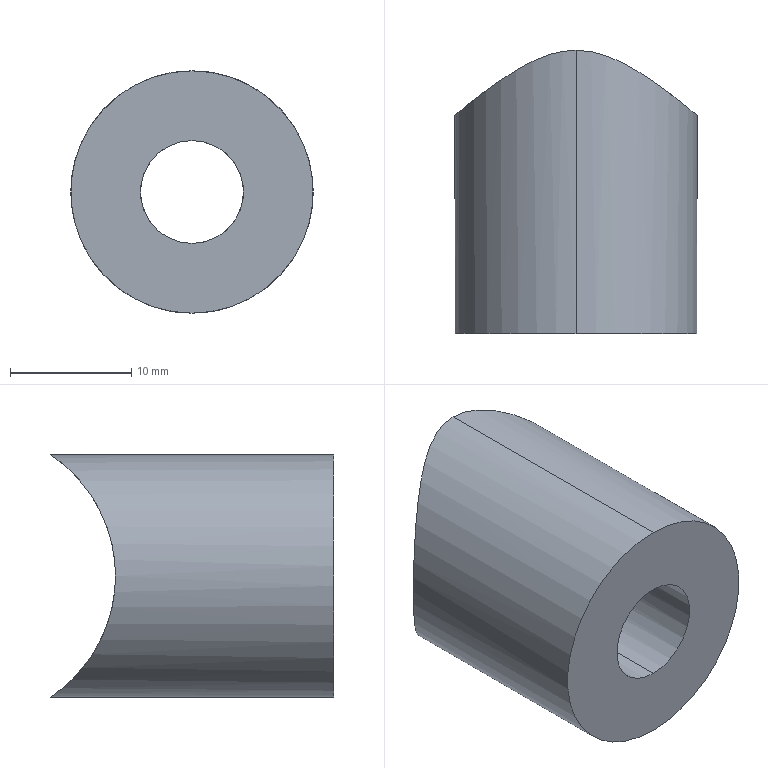Part | SolidWorks | features 3DProfileFeature 1, Extrusion 1, HoleWzd 1 | 1 solid | 7 faces | box 20 x 23.367 x 20 mm | volume 4988 mm3 | cylinder 6 | plane 1 | commonest cylinder face diameters 8.5 x2 20 x2 24 x2
STEP:
#1=CARTESIAN_POINT('',(-608.25,85.2,0.));
#2=VERTEX_POINT('',#1);
#3=CARTESIAN_POINT('',(-604.,85.978,4.25));
#4=VERTEX_POINT('',#3);
#5=CARTESIAN_POINT('',(-608.25,85.2,0.));
#6=CARTESIAN_POINT('',(-608.25,85.2,0.2798));
#7=CARTESIAN_POINT('',(-608.222,85.21,0.5639));
#8=CARTESIAN_POINT('',(-608.112,85.248,1.111));
#9=CARTESIAN_POINT('',(-608.031,85.276,1.377));
#10=CARTESIAN_POINT('',(-607.815,85.348,1.895));
#11=CARTESIAN_POINT('',(-607.683,85.39,2.139));
#12=CARTESIAN_POINT('',(-607.376,85.482,2.597));
#13=CARTESIAN_POINT('',(-607.198,85.533,2.813));
#14=CARTESIAN_POINT('',(-606.807,85.634,3.203));
#15=CARTESIAN_POINT('',(-606.595,85.684,3.377));
#16=CARTESIAN_POINT('',(-606.136,85.779,3.685));
#17=CARTESIAN_POINT('',(-605.887,85.823,3.818));
#18=CARTESIAN_POINT('',(-605.376,85.897,4.03));
#19=CARTESIAN_POINT('',(-605.111,85.926,4.112));
#20=CARTESIAN_POINT('',(-604.56,85.967,4.222));
#21=CARTESIAN_POINT('',(-604.279,85.978,4.25));
#22=CARTESIAN_POINT('',(-604.,85.978,4.25));
#23=B_SPLINE_CURVE_WITH_KNOTS('',3,(#5,#6,#7,#8,#9,#10,#11,#12,#13,#14,#15,#16,#17,#18,#19,#20,#21,#22),.UNSPECIFIED.,.F.,.F.,(4,2,2,2,2,2,2,2,4),(0.0067,0.007537,0.008374,0.009211,0.01005,0.01089,0.01172,0.01256,0.0134),.UNSPECIFIED.);
#24=EDGE_CURVE('',#2,#4,#23,.T.);
#25=ORIENTED_EDGE('',*,*,#24,.T.);
#26=CARTESIAN_POINT('',(-604.,67.2,4.25));
#27=VERTEX_POINT('',#26);
#28=CARTESIAN_POINT('',(-604.,67.2,4.25));
#29=DIRECTION('',(0.,-1.,0.));
#30=VECTOR('',#29,1000.);
#31=LINE('',#28,#30);
#32=EDGE_CURVE('',#4,#27,#31,.T.);
#33=ORIENTED_EDGE('',*,*,#32,.T.);
#34=CARTESIAN_POINT('',(-604.,67.2,-4.25));
#35=VERTEX_POINT('',#34);
#36=CARTESIAN_POINT('',(-604.,67.2,0.));
#37=DIRECTION('',(0.,-1.,0.));
#38=DIRECTION('',(0.,0.,-1.));
#39=AXIS2_PLACEMENT_3D('',#36,#37,#38);
#40=CIRCLE('',#39,4.25);
#41=EDGE_CURVE('',#27,#35,#40,.T.);
#42=ORIENTED_EDGE('',*,*,#41,.T.);
#43=CARTESIAN_POINT('',(-604.,85.978,-4.25));
#44=VERTEX_POINT('',#43);
#45=CARTESIAN_POINT('',(-604.,67.2,-4.25));
#46=DIRECTION('',(0.,-1.,0.));
#47=VECTOR('',#46,1000.);
#48=LINE('',#45,#47);
#49=EDGE_CURVE('',#44,#35,#48,.T.);
#50=ORIENTED_EDGE('',*,*,#49,.F.);
#51=CARTESIAN_POINT('',(-604.,85.978,-4.25));
#52=CARTESIAN_POINT('',(-604.283,85.978,-4.25));
#53=CARTESIAN_POINT('',(-604.562,85.967,-4.222));
#54=CARTESIAN_POINT('',(-605.108,85.927,-4.112));
#55=CARTESIAN_POINT('',(-605.379,85.896,-4.03));
#56=CARTESIAN_POINT('',(-605.893,85.822,-3.815));
#57=CARTESIAN_POINT('',(-606.136,85.779,-3.685));
#58=CARTESIAN_POINT('',(-606.596,85.684,-3.376));
#59=CARTESIAN_POINT('',(-606.812,85.632,-3.199));
#60=CARTESIAN_POINT('',(-607.201,85.532,-2.81));
#61=CARTESIAN_POINT('',(-607.376,85.482,-2.597));
#62=CARTESIAN_POINT('',(-607.687,85.389,-2.133));
#63=CARTESIAN_POINT('',(-607.817,85.347,-1.889));
#64=CARTESIAN_POINT('',(-608.03,85.277,-1.378));
#65=CARTESIAN_POINT('',(-608.113,85.248,-1.108));
#66=CARTESIAN_POINT('',(-608.223,85.21,-0.5575));
#67=CARTESIAN_POINT('',(-608.25,85.2,-0.28));
#68=CARTESIAN_POINT('',(-608.25,85.2,0.));
#69=B_SPLINE_CURVE_WITH_KNOTS('',3,(#51,#52,#53,#54,#55,#56,#57,#58,#59,#60,#61,#62,#63,#64,#65,#66,#67,#68),.UNSPECIFIED.,.F.,.F.,(4,2,2,2,2,2,2,2,4),(0.,0.0008375,0.001675,0.002513,0.00335,0.004188,0.005025,0.005863,0.0067),.UNSPECIFIED.);
#70=EDGE_CURVE('',#44,#2,#69,.T.);
#71=ORIENTED_EDGE('',*,*,#70,.T.);
#72=EDGE_LOOP('',(#25,#33,#42,#50,#71));
#73=FACE_OUTER_BOUND('',#72,.T.);
#74=CARTESIAN_POINT('',(-604.,67.2,0.));
#75=DIRECTION('',(0.,-1.,0.));
#76=DIRECTION('',(0.,0.,-1.));
#77=AXIS2_PLACEMENT_3D('',#74,#75,#76);
#78=CYLINDRICAL_SURFACE('',#77,4.25);
#79=ADVANCED_FACE('',(#73),#78,.F.);
#80=CARTESIAN_POINT('',(-604.,90.567,10.));
#81=VERTEX_POINT('',#80);
#82=CARTESIAN_POINT('',(-594.,85.2,0.));
#83=VERTEX_POINT('',#82);
#84=CARTESIAN_POINT('',(-604.,90.567,10.));
#85=CARTESIAN_POINT('',(-603.65,90.567,10.));
#86=CARTESIAN_POINT('',(-603.302,90.539,9.982));
#87=CARTESIAN_POINT('',(-602.614,90.432,9.91));
#88=CARTESIAN_POINT('',(-602.27,90.352,9.855));
#89=CARTESIAN_POINT('',(-601.282,90.059,9.647));
#90=CARTESIAN_POINT('',(-600.666,89.793,9.449));
#91=CARTESIAN_POINT('',(-599.491,89.195,8.948));
#92=CARTESIAN_POINT('',(-598.949,88.872,8.652));
#93=CARTESIAN_POINT('',(-597.929,88.216,7.97));
#94=CARTESIAN_POINT('',(-597.45,87.883,7.582));
#95=CARTESIAN_POINT('',(-596.558,87.236,6.709));
#96=CARTESIAN_POINT('',(-596.154,86.929,6.233));
#97=CARTESIAN_POINT('',(-595.612,86.507,5.454));
#98=CARTESIAN_POINT('',(-595.442,86.373,5.183));
#99=CARTESIAN_POINT('',(-595.124,86.12,4.617));
#100=CARTESIAN_POINT('',(-594.976,86.,4.321));
#101=CARTESIAN_POINT('',(-594.571,85.673,3.399));
#102=CARTESIAN_POINT('',(-594.362,85.5,2.755));
#103=CARTESIAN_POINT('',(-594.147,85.322,1.741));
#104=CARTESIAN_POINT('',(-594.091,85.276,1.392));
#105=CARTESIAN_POINT('',(-594.018,85.215,0.6965));
#106=CARTESIAN_POINT('',(-594.,85.2,0.3484));
#107=CARTESIAN_POINT('',(-594.,85.2,0.));
#108=B_SPLINE_CURVE_WITH_KNOTS('',3,(#84,#85,#86,#87,#88,#89,#90,#91,#92,#93,#94,#95,#96,#97,#98,#99,#100,#101,#102,#103,#104,#105,#106,#107),.UNSPECIFIED.,.F.,.F.,(4,2,2,2,2,2,2,2,2,2,2,4),(0.03345,0.0345,0.03555,0.03764,0.03974,0.04183,0.04392,0.04497,0.04602,0.04811,0.04916,0.0502),.UNSPECIFIED.);
#109=EDGE_CURVE('',#81,#83,#108,.T.);
#110=ORIENTED_EDGE('',*,*,#109,.T.);
#111=CARTESIAN_POINT('',(-599.75,85.2,0.));
#112=VERTEX_POINT('',#111);
#113=CARTESIAN_POINT('',(-550.186,85.2,0.));
#114=DIRECTION('',(-1.,0.,0.));
#115=VECTOR('',#114,1000.);
#116=LINE('',#113,#115);
#117=EDGE_CURVE('',#83,#112,#116,.T.);
#118=ORIENTED_EDGE('',*,*,#117,.T.);
#119=CARTESIAN_POINT('',(-604.,85.978,4.25));
#120=CARTESIAN_POINT('',(-603.721,85.978,4.25));
#121=CARTESIAN_POINT('',(-603.44,85.967,4.222));
#122=CARTESIAN_POINT('',(-602.889,85.926,4.112));
#123=CARTESIAN_POINT('',(-602.623,85.896,4.03));
#124=CARTESIAN_POINT('',(-602.11,85.823,3.817));
#125=CARTESIAN_POINT('',(-601.862,85.778,3.683));
#126=CARTESIAN_POINT('',(-601.404,85.684,3.376));
#127=CARTESIAN_POINT('',(-601.191,85.633,3.202));
#128=CARTESIAN_POINT('',(-600.799,85.532,2.809));
#129=CARTESIAN_POINT('',(-600.623,85.482,2.595));
#130=CARTESIAN_POINT('',(-600.317,85.39,2.138));
#131=CARTESIAN_POINT('',(-600.184,85.347,1.891));
#132=CARTESIAN_POINT('',(-599.969,85.276,1.376));
#133=CARTESIAN_POINT('',(-599.888,85.248,1.11));
#134=CARTESIAN_POINT('',(-599.778,85.21,0.5641));
#135=CARTESIAN_POINT('',(-599.75,85.2,0.28));
#136=CARTESIAN_POINT('',(-599.75,85.2,0.));
#137=B_SPLINE_CURVE_WITH_KNOTS('',3,(#119,#120,#121,#122,#123,#124,#125,#126,#127,#128,#129,#130,#131,#132,#133,#134,#135,#136),.UNSPECIFIED.,.F.,.F.,(4,2,2,2,2,2,2,2,4),(0.0134,0.01423,0.01507,0.01591,0.01674,0.01758,0.01842,0.01926,0.02009),.UNSPECIFIED.);
#138=EDGE_CURVE('',#4,#112,#137,.T.);
#139=ORIENTED_EDGE('',*,*,#138,.F.);
#140=ORIENTED_EDGE('',*,*,#24,.F.);
#141=CARTESIAN_POINT('',(-614.,85.2,0.));
#142=VERTEX_POINT('',#141);
#143=CARTESIAN_POINT('',(-550.186,85.2,0.));
#144=DIRECTION('',(-1.,0.,0.));
#145=VECTOR('',#144,1000.);
#146=LINE('',#143,#145);
#147=EDGE_CURVE('',#2,#142,#146,.T.);
#148=ORIENTED_EDGE('',*,*,#147,.T.);
#149=CARTESIAN_POINT('',(-614.,85.2,0.));
#150=CARTESIAN_POINT('',(-614.,85.2,0.3474));
#151=CARTESIAN_POINT('',(-613.982,85.215,0.6944));
#152=CARTESIAN_POINT('',(-613.909,85.275,1.388));
#153=CARTESIAN_POINT('',(-613.854,85.321,1.735));
#154=CARTESIAN_POINT('',(-613.64,85.499,2.748));
#155=CARTESIAN_POINT('',(-613.431,85.671,3.392));
#156=CARTESIAN_POINT('',(-612.894,86.106,4.621));
#157=CARTESIAN_POINT('',(-612.574,86.362,5.186));
#158=CARTESIAN_POINT('',(-612.026,86.788,5.974));
#159=CARTESIAN_POINT('',(-611.831,86.938,6.227));
#160=CARTESIAN_POINT('',(-611.424,87.245,6.707));
#161=CARTESIAN_POINT('',(-611.212,87.403,6.935));
#162=CARTESIAN_POINT('',(-610.55,87.883,7.582));
#163=CARTESIAN_POINT('',(-610.076,88.213,7.967));
#164=CARTESIAN_POINT('',(-609.308,88.707,8.481));
#165=CARTESIAN_POINT('',(-609.041,88.872,8.642));
#166=CARTESIAN_POINT('',(-608.493,89.192,8.939));
#167=CARTESIAN_POINT('',(-608.211,89.347,9.075));
#168=CARTESIAN_POINT('',(-607.631,89.642,9.323));
#169=CARTESIAN_POINT('',(-607.331,89.783,9.434));
#170=CARTESIAN_POINT('',(-606.711,90.04,9.631));
#171=CARTESIAN_POINT('',(-606.387,90.157,9.717));
#172=CARTESIAN_POINT('',(-605.729,90.352,9.855));
#173=CARTESIAN_POINT('',(-605.393,90.431,9.909));
#174=CARTESIAN_POINT('',(-604.705,90.538,9.981));
#175=CARTESIAN_POINT('',(-604.35,90.567,10.));
#176=CARTESIAN_POINT('',(-604.,90.567,10.));
#177=B_SPLINE_CURVE_WITH_KNOTS('',3,(#149,#150,#151,#152,#153,#154,#155,#156,#157,#158,#159,#160,#161,#162,#163,#164,#165,#166,#167,#168,#169,#170,#171,#172,#173,#174,#175,#176),.UNSPECIFIED.,.F.,.F.,(4,2,2,2,2,2,2,2,2,2,2,2,2,4),(0.01674,0.01778,0.01883,0.02092,0.02301,0.02405,0.0251,0.02719,0.02823,0.02927,0.03032,0.03136,0.03241,0.03345),.UNSPECIFIED.);
#178=EDGE_CURVE('',#142,#81,#177,.T.);
#179=ORIENTED_EDGE('',*,*,#178,.T.);
#180=EDGE_LOOP('',(#110,#118,#139,#140,#148,#179));
#181=FACE_OUTER_BOUND('',#180,.T.);
#182=CARTESIAN_POINT('',(-550.186,97.2,0.));
#183=DIRECTION('',(-1.,0.,0.));
#184=DIRECTION('',(0.,-1.,0.));
#185=AXIS2_PLACEMENT_3D('',#182,#183,#184);
#186=CYLINDRICAL_SURFACE('',#185,12.);
#187=ADVANCED_FACE('',(#181),#186,.F.);
#188=ORIENTED_EDGE('',*,*,#109,.F.);
#189=CARTESIAN_POINT('',(-604.,67.2,10.));
#190=VERTEX_POINT('',#189);
#191=CARTESIAN_POINT('',(-604.,109.201,10.));
#192=DIRECTION('',(0.,-1.,0.));
#193=VECTOR('',#192,1000.);
#194=LINE('',#191,#193);
#195=EDGE_CURVE('',#81,#190,#194,.T.);
#196=ORIENTED_EDGE('',*,*,#195,.T.);
#197=CARTESIAN_POINT('',(-604.,67.2,-10.));
#198=VERTEX_POINT('',#197);
#199=CARTESIAN_POINT('',(-604.,67.2,0.));
#200=DIRECTION('',(0.,1.,0.));
#201=DIRECTION('',(0.,0.,1.));
#202=AXIS2_PLACEMENT_3D('',#199,#200,#201);
#203=CIRCLE('',#202,10.);
#204=EDGE_CURVE('',#190,#198,#203,.T.);
#205=ORIENTED_EDGE('',*,*,#204,.T.);
#206=CARTESIAN_POINT('',(-604.,90.567,-10.));
#207=VERTEX_POINT('',#206);
#208=CARTESIAN_POINT('',(-604.,109.201,-10.));
#209=DIRECTION('',(0.,-1.,0.));
#210=VECTOR('',#209,1000.);
#211=LINE('',#208,#210);
#212=EDGE_CURVE('',#207,#198,#211,.T.);
#213=ORIENTED_EDGE('',*,*,#212,.F.);
#214=CARTESIAN_POINT('',(-594.,85.2,0.));
#215=CARTESIAN_POINT('',(-594.,85.2,-0.3472));
#216=CARTESIAN_POINT('',(-594.018,85.215,-0.6948));
#217=CARTESIAN_POINT('',(-594.091,85.276,-1.39));
#218=CARTESIAN_POINT('',(-594.146,85.321,-1.737));
#219=CARTESIAN_POINT('',(-594.289,85.44,-2.41));
#220=CARTESIAN_POINT('',(-594.377,85.512,-2.74));
#221=CARTESIAN_POINT('',(-594.584,85.682,-3.384));
#222=CARTESIAN_POINT('',(-594.704,85.781,-3.702));
#223=CARTESIAN_POINT('',(-595.106,86.106,-4.62));
#224=CARTESIAN_POINT('',(-595.425,86.362,-5.185));
#225=CARTESIAN_POINT('',(-595.974,86.789,-5.974));
#226=CARTESIAN_POINT('',(-596.17,86.938,-6.228));
#227=CARTESIAN_POINT('',(-596.576,87.245,-6.706));
#228=CARTESIAN_POINT('',(-596.787,87.402,-6.933));
#229=CARTESIAN_POINT('',(-597.448,87.881,-7.58));
#230=CARTESIAN_POINT('',(-597.923,88.212,-7.965));
#231=CARTESIAN_POINT('',(-598.692,88.707,-8.481));
#232=CARTESIAN_POINT('',(-598.959,88.872,-8.642));
#233=CARTESIAN_POINT('',(-599.506,89.191,-8.939));
#234=CARTESIAN_POINT('',(-599.787,89.346,-9.075));
#235=CARTESIAN_POINT('',(-600.367,89.641,-9.322));
#236=CARTESIAN_POINT('',(-600.666,89.781,-9.433));
#237=CARTESIAN_POINT('',(-601.287,90.039,-9.63));
#238=CARTESIAN_POINT('',(-601.61,90.156,-9.716));
#239=CARTESIAN_POINT('',(-602.268,90.352,-9.855));
#240=CARTESIAN_POINT('',(-602.604,90.43,-9.908));
#241=CARTESIAN_POINT('',(-603.292,90.538,-9.981));
#242=CARTESIAN_POINT('',(-603.646,90.567,-10.));
#243=CARTESIAN_POINT('',(-604.,90.567,-10.));
#244=B_SPLINE_CURVE_WITH_KNOTS('',3,(#214,#215,#216,#217,#218,#219,#220,#221,#222,#223,#224,#225,#226,#227,#228,#229,#230,#231,#232,#233,#234,#235,#236,#237,#238,#239,#240,#241,#242,#243),.UNSPECIFIED.,.F.,.F.,(4,2,2,2,2,2,2,2,2,2,2,2,2,2,4),(0.0502,0.05125,0.05229,0.05333,0.05438,0.05646,0.05751,0.05855,0.06064,0.06168,0.06272,0.06377,0.06481,0.06586,0.0669),.UNSPECIFIED.);
#245=EDGE_CURVE('',#83,#207,#244,.T.);
#246=ORIENTED_EDGE('',*,*,#245,.F.);
#247=EDGE_LOOP('',(#188,#196,#205,#213,#246));
#248=FACE_OUTER_BOUND('',#247,.T.);
#249=CARTESIAN_POINT('',(-604.,109.201,0.));
#250=DIRECTION('',(0.,-1.,0.));
#251=DIRECTION('',(0.,0.,-1.));
#252=AXIS2_PLACEMENT_3D('',#249,#250,#251);
#253=CYLINDRICAL_SURFACE('',#252,10.);
#254=ADVANCED_FACE('',(#248),#253,.T.);
#255=CARTESIAN_POINT('',(-604.,67.2,0.));
#256=DIRECTION('',(0.,-1.,0.));
#257=DIRECTION('',(0.,0.,-1.));
#258=AXIS2_PLACEMENT_3D('',#255,#256,#257);
#259=CIRCLE('',#258,4.25);
#260=EDGE_CURVE('',#35,#27,#259,.T.);
#261=ORIENTED_EDGE('',*,*,#260,.F.);
#262=ORIENTED_EDGE('',*,*,#41,.F.);
#263=EDGE_LOOP('',(#261,#262));
#264=FACE_BOUND('',#263,.T.);
#265=CARTESIAN_POINT('',(-604.,67.2,0.));
#266=DIRECTION('',(0.,1.,0.));
#267=DIRECTION('',(0.,0.,1.));
#268=AXIS2_PLACEMENT_3D('',#265,#266,#267);
#269=CIRCLE('',#268,10.);
#270=EDGE_CURVE('',#198,#190,#269,.T.);
#271=ORIENTED_EDGE('',*,*,#270,.F.);
#272=ORIENTED_EDGE('',*,*,#204,.F.);
#273=EDGE_LOOP('',(#271,#272));
#274=FACE_OUTER_BOUND('',#273,.T.);
#275=CARTESIAN_POINT('',(-604.,67.2,0.));
#276=DIRECTION('',(0.,1.,0.));
#277=DIRECTION('',(0.,0.,1.));
#278=AXIS2_PLACEMENT_3D('',#275,#276,#277);
#279=PLANE('',#278);
#280=ADVANCED_FACE('',(#264,#274),#279,.F.);
#281=ORIENTED_EDGE('',*,*,#195,.F.);
#282=ORIENTED_EDGE('',*,*,#178,.F.);
#283=CARTESIAN_POINT('',(-604.,90.567,-10.));
#284=CARTESIAN_POINT('',(-604.709,90.567,-10.));
#285=CARTESIAN_POINT('',(-605.393,90.452,-9.926));
#286=CARTESIAN_POINT('',(-606.722,90.058,-9.646));
#287=CARTESIAN_POINT('',(-607.337,89.792,-9.448));
#288=CARTESIAN_POINT('',(-608.21,89.348,-9.076));
#289=CARTESIAN_POINT('',(-608.494,89.191,-8.939));
#290=CARTESIAN_POINT('',(-609.043,88.87,-8.641));
#291=CARTESIAN_POINT('',(-609.307,88.707,-8.481));
#292=CARTESIAN_POINT('',(-610.073,88.215,-7.969));
#293=CARTESIAN_POINT('',(-610.547,87.885,-7.584));
#294=CARTESIAN_POINT('',(-611.432,87.243,-6.719));
#295=CARTESIAN_POINT('',(-611.845,86.929,-6.234));
#296=CARTESIAN_POINT('',(-612.573,86.363,-5.188));
#297=CARTESIAN_POINT('',(-612.892,86.108,-4.624));
#298=CARTESIAN_POINT('',(-613.295,85.781,-3.704));
#299=CARTESIAN_POINT('',(-613.415,85.683,-3.387));
#300=CARTESIAN_POINT('',(-613.623,85.513,-2.743));
#301=CARTESIAN_POINT('',(-613.711,85.44,-2.413));
#302=CARTESIAN_POINT('',(-613.853,85.322,-1.74));
#303=CARTESIAN_POINT('',(-613.909,85.276,-1.394));
#304=CARTESIAN_POINT('',(-613.982,85.215,-0.6962));
#305=CARTESIAN_POINT('',(-614.,85.2,-0.3479));
#306=CARTESIAN_POINT('',(-614.,85.2,0.));
#307=B_SPLINE_CURVE_WITH_KNOTS('',3,(#283,#284,#285,#286,#287,#288,#289,#290,#291,#292,#293,#294,#295,#296,#297,#298,#299,#300,#301,#302,#303,#304,#305,#306),.UNSPECIFIED.,.F.,.F.,(4,2,2,2,2,2,2,2,2,2,2,4),(0.,0.002092,0.004185,0.005231,0.006277,0.008369,0.01046,0.01255,0.0136,0.01465,0.01569,0.01674),.UNSPECIFIED.);
#308=EDGE_CURVE('',#207,#142,#307,.T.);
#309=ORIENTED_EDGE('',*,*,#308,.F.);
#310=ORIENTED_EDGE('',*,*,#212,.T.);
#311=ORIENTED_EDGE('',*,*,#270,.T.);
#312=EDGE_LOOP('',(#281,#282,#309,#310,#311));
#313=FACE_OUTER_BOUND('',#312,.T.);
#314=CARTESIAN_POINT('',(-604.,109.201,0.));
#315=DIRECTION('',(0.,-1.,0.));
#316=DIRECTION('',(0.,0.,-1.));
#317=AXIS2_PLACEMENT_3D('',#314,#315,#316);
#318=CYLINDRICAL_SURFACE('',#317,10.);
#319=ADVANCED_FACE('',(#313),#318,.T.);
#320=ORIENTED_EDGE('',*,*,#117,.F.);
#321=ORIENTED_EDGE('',*,*,#245,.T.);
#322=ORIENTED_EDGE('',*,*,#308,.T.);
#323=ORIENTED_EDGE('',*,*,#147,.F.);
#324=ORIENTED_EDGE('',*,*,#70,.F.);
#325=CARTESIAN_POINT('',(-599.75,85.2,0.));
#326=CARTESIAN_POINT('',(-599.75,85.2,-0.2801));
#327=CARTESIAN_POINT('',(-599.777,85.21,-0.5578));
#328=CARTESIAN_POINT('',(-599.888,85.248,-1.109));
#329=CARTESIAN_POINT('',(-599.97,85.277,-1.379));
#330=CARTESIAN_POINT('',(-600.184,85.347,-1.891));
#331=CARTESIAN_POINT('',(-600.316,85.39,-2.137));
#332=CARTESIAN_POINT('',(-600.626,85.482,-2.599));
#333=CARTESIAN_POINT('',(-600.801,85.532,-2.811));
#334=CARTESIAN_POINT('',(-601.19,85.633,-3.201));
#335=CARTESIAN_POINT('',(-601.407,85.684,-3.379));
#336=CARTESIAN_POINT('',(-601.866,85.779,-3.686));
#337=CARTESIAN_POINT('',(-602.109,85.822,-3.816));
#338=CARTESIAN_POINT('',(-602.623,85.897,-4.03));
#339=CARTESIAN_POINT('',(-602.893,85.927,-4.113));
#340=CARTESIAN_POINT('',(-603.439,85.967,-4.222));
#341=CARTESIAN_POINT('',(-603.717,85.978,-4.25));
#342=CARTESIAN_POINT('',(-604.,85.978,-4.25));
#343=B_SPLINE_CURVE_WITH_KNOTS('',3,(#325,#326,#327,#328,#329,#330,#331,#332,#333,#334,#335,#336,#337,#338,#339,#340,#341,#342),.UNSPECIFIED.,.F.,.F.,(4,2,2,2,2,2,2,2,4),(0.02009,0.02093,0.02177,0.0226,0.02344,0.02428,0.02512,0.02595,0.02679),.UNSPECIFIED.);
#344=EDGE_CURVE('',#112,#44,#343,.T.);
#345=ORIENTED_EDGE('',*,*,#344,.F.);
#346=EDGE_LOOP('',(#320,#321,#322,#323,#324,#345));
#347=FACE_OUTER_BOUND('',#346,.T.);
#348=CARTESIAN_POINT('',(-550.186,97.2,0.));
#349=DIRECTION('',(-1.,0.,0.));
#350=DIRECTION('',(0.,-1.,0.));
#351=AXIS2_PLACEMENT_3D('',#348,#349,#350);
#352=CYLINDRICAL_SURFACE('',#351,12.);
#353=ADVANCED_FACE('',(#347),#352,.F.);
#354=ORIENTED_EDGE('',*,*,#32,.F.);
#355=ORIENTED_EDGE('',*,*,#138,.T.);
#356=ORIENTED_EDGE('',*,*,#344,.T.);
#357=ORIENTED_EDGE('',*,*,#49,.T.);
#358=ORIENTED_EDGE('',*,*,#260,.T.);
#359=EDGE_LOOP('',(#354,#355,#356,#357,#358));
#360=FACE_OUTER_BOUND('',#359,.T.);
#361=CARTESIAN_POINT('',(-604.,67.2,0.));
#362=DIRECTION('',(0.,-1.,0.));
#363=DIRECTION('',(0.,0.,-1.));
#364=AXIS2_PLACEMENT_3D('',#361,#362,#363);
#365=CYLINDRICAL_SURFACE('',#364,4.25);
#366=ADVANCED_FACE('',(#360),#365,.F.);
#367=CLOSED_SHELL('',(#79,#187,#254,#280,#319,#353,#366));
#368=MANIFOLD_SOLID_BREP('',#367);
#369=CARTESIAN_POINT('',(0.,0.,0.));
#370=DIRECTION('',(0.,0.,1.));
#371=DIRECTION('',(1.,0.,0.));
#372=AXIS2_PLACEMENT_3D('',#369,#370,#371);
#373=(LENGTH_UNIT()NAMED_UNIT(*)SI_UNIT(.MILLI.,.METRE.));
#374=UNCERTAINTY_MEASURE_WITH_UNIT(LENGTH_MEASURE(0.00001),#373,'','');
#375=(NAMED_UNIT(*)PLANE_ANGLE_UNIT()SI_UNIT($,.RADIAN.));
#376=(NAMED_UNIT(*)SI_UNIT($,.STERADIAN.)SOLID_ANGLE_UNIT());
#377=(GEOMETRIC_REPRESENTATION_CONTEXT(3)GLOBAL_UNCERTAINTY_ASSIGNED_CONTEXT((#374))GLOBAL_UNIT_ASSIGNED_CONTEXT((#373,#375,#376))REPRESENTATION_CONTEXT('',''));
#378=ADVANCED_BREP_SHAPE_REPRESENTATION('',(#368,#372),#377);